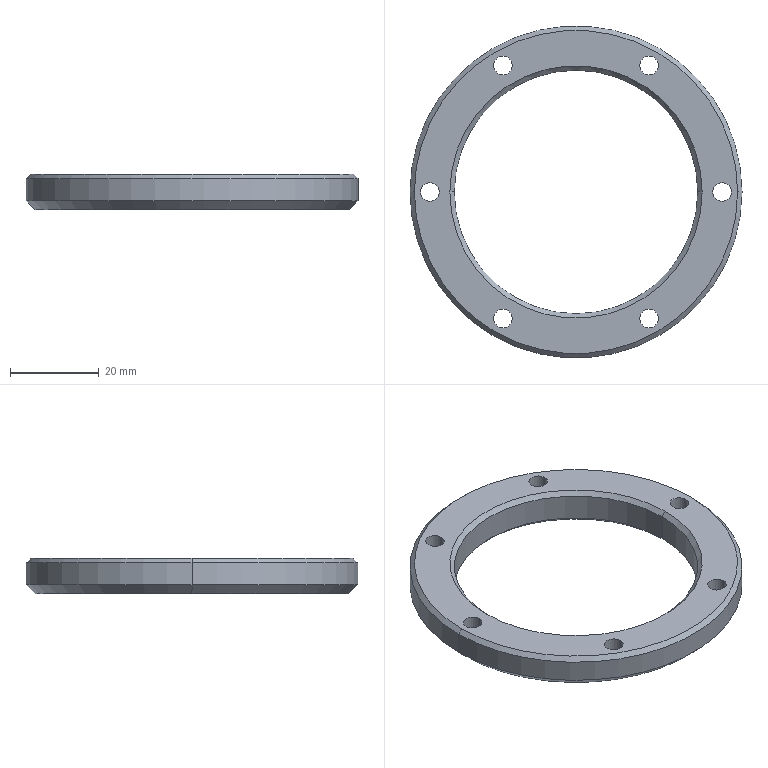Part | STEP file | 10000020571swp000-1 | 1 solid | 26 faces | box 75 x 75 x 8 mm | volume 14917 mm3 | cylinder 16 | cone 8 | plane 2 | commonest cylinder face diameters 4.2 x12 55 x2 75 x2
STEP:
#1=CARTESIAN_POINT('',(-35.5,0.,0.));
#2=VERTEX_POINT('',#1);
#3=CARTESIAN_POINT('',(35.5,0.,0.));
#4=VERTEX_POINT('',#3);
#5=CARTESIAN_POINT('',(0.,0.,0.));
#6=DIRECTION('',(0.,0.,-1.));
#7=DIRECTION('',(1.,0.,0.));
#8=AXIS2_PLACEMENT_3D('',#5,#6,#7);
#9=CIRCLE('',#8,35.5);
#10=EDGE_CURVE('',#2,#4,#9,.T.);
#11=ORIENTED_EDGE('',*,*,#10,.F.);
#12=CARTESIAN_POINT('',(-37.5,0.,2.));
#13=VERTEX_POINT('',#12);
#14=CARTESIAN_POINT('',(-37.5,0.,2.));
#15=DIRECTION('',(-0.7071,0.,0.7071));
#16=VECTOR('',#15,1000.);
#17=LINE('',#14,#16);
#18=EDGE_CURVE('',#2,#13,#17,.T.);
#19=ORIENTED_EDGE('',*,*,#18,.T.);
#20=CARTESIAN_POINT('',(37.5,0.,2.));
#21=VERTEX_POINT('',#20);
#22=CARTESIAN_POINT('',(0.,0.,2.));
#23=DIRECTION('',(0.,0.,1.));
#24=DIRECTION('',(1.,0.,0.));
#25=AXIS2_PLACEMENT_3D('',#22,#23,#24);
#26=CIRCLE('',#25,37.5);
#27=EDGE_CURVE('',#21,#13,#26,.T.);
#28=ORIENTED_EDGE('',*,*,#27,.F.);
#29=CARTESIAN_POINT('',(37.5,0.,2.));
#30=DIRECTION('',(0.7071,0.,0.7071));
#31=VECTOR('',#30,1000.);
#32=LINE('',#29,#31);
#33=EDGE_CURVE('',#4,#21,#32,.T.);
#34=ORIENTED_EDGE('',*,*,#33,.F.);
#35=EDGE_LOOP('',(#11,#19,#28,#34));
#36=FACE_OUTER_BOUND('',#35,.T.);
#37=CARTESIAN_POINT('',(0.,0.,2.));
#38=DIRECTION('',(0.,0.,1.));
#39=DIRECTION('',(1.,0.,0.));
#40=AXIS2_PLACEMENT_3D('',#37,#38,#39);
#41=CONICAL_SURFACE('',#40,37.5,0.7854);
#42=ADVANCED_FACE('',(#36),#41,.T.);
#43=CARTESIAN_POINT('',(-27.5,0.,7.));
#44=VERTEX_POINT('',#43);
#45=CARTESIAN_POINT('',(27.5,0.,7.));
#46=VERTEX_POINT('',#45);
#47=CARTESIAN_POINT('',(0.,0.,7.));
#48=DIRECTION('',(0.,0.,1.));
#49=DIRECTION('',(1.,0.,0.));
#50=AXIS2_PLACEMENT_3D('',#47,#48,#49);
#51=CIRCLE('',#50,27.5);
#52=EDGE_CURVE('',#44,#46,#51,.T.);
#53=ORIENTED_EDGE('',*,*,#52,.F.);
#54=CARTESIAN_POINT('',(-28.5,0.,8.));
#55=VERTEX_POINT('',#54);
#56=CARTESIAN_POINT('',(-27.5,0.,7.));
#57=DIRECTION('',(-0.7071,0.,0.7071));
#58=VECTOR('',#57,1000.);
#59=LINE('',#56,#58);
#60=EDGE_CURVE('',#44,#55,#59,.T.);
#61=ORIENTED_EDGE('',*,*,#60,.T.);
#62=CARTESIAN_POINT('',(28.5,0.,8.));
#63=VERTEX_POINT('',#62);
#64=CARTESIAN_POINT('',(0.,0.,8.));
#65=DIRECTION('',(0.,0.,-1.));
#66=DIRECTION('',(1.,0.,0.));
#67=AXIS2_PLACEMENT_3D('',#64,#65,#66);
#68=CIRCLE('',#67,28.5);
#69=EDGE_CURVE('',#63,#55,#68,.T.);
#70=ORIENTED_EDGE('',*,*,#69,.F.);
#71=CARTESIAN_POINT('',(27.5,0.,7.));
#72=DIRECTION('',(0.7071,0.,0.7071));
#73=VECTOR('',#72,1000.);
#74=LINE('',#71,#73);
#75=EDGE_CURVE('',#46,#63,#74,.T.);
#76=ORIENTED_EDGE('',*,*,#75,.F.);
#77=EDGE_LOOP('',(#53,#61,#70,#76));
#78=FACE_OUTER_BOUND('',#77,.T.);
#79=CARTESIAN_POINT('',(0.,0.,7.));
#80=DIRECTION('',(0.,0.,1.));
#81=DIRECTION('',(1.,0.,0.));
#82=AXIS2_PLACEMENT_3D('',#79,#80,#81);
#83=CONICAL_SURFACE('',#82,27.5,0.7854);
#84=ADVANCED_FACE('',(#78),#83,.F.);
#85=CARTESIAN_POINT('',(27.5,0.,1.));
#86=VERTEX_POINT('',#85);
#87=CARTESIAN_POINT('',(-27.5,0.,1.));
#88=VERTEX_POINT('',#87);
#89=CARTESIAN_POINT('',(0.,0.,1.));
#90=DIRECTION('',(0.,0.,-1.));
#91=DIRECTION('',(1.,0.,0.));
#92=AXIS2_PLACEMENT_3D('',#89,#90,#91);
#93=CIRCLE('',#92,27.5);
#94=EDGE_CURVE('',#86,#88,#93,.T.);
#95=ORIENTED_EDGE('',*,*,#94,.F.);
#96=CARTESIAN_POINT('',(28.5,0.,0.));
#97=VERTEX_POINT('',#96);
#98=CARTESIAN_POINT('',(28.5,0.,0.));
#99=DIRECTION('',(0.7071,0.,-0.7071));
#100=VECTOR('',#99,1000.);
#101=LINE('',#98,#100);
#102=EDGE_CURVE('',#86,#97,#101,.T.);
#103=ORIENTED_EDGE('',*,*,#102,.T.);
#104=CARTESIAN_POINT('',(-28.5,0.,0.));
#105=VERTEX_POINT('',#104);
#106=CARTESIAN_POINT('',(0.,0.,0.));
#107=DIRECTION('',(0.,0.,1.));
#108=DIRECTION('',(1.,0.,0.));
#109=AXIS2_PLACEMENT_3D('',#106,#107,#108);
#110=CIRCLE('',#109,28.5);
#111=EDGE_CURVE('',#105,#97,#110,.T.);
#112=ORIENTED_EDGE('',*,*,#111,.F.);
#113=CARTESIAN_POINT('',(-28.5,0.,0.));
#114=DIRECTION('',(-0.7071,0.,-0.7071));
#115=VECTOR('',#114,1000.);
#116=LINE('',#113,#115);
#117=EDGE_CURVE('',#88,#105,#116,.T.);
#118=ORIENTED_EDGE('',*,*,#117,.F.);
#119=EDGE_LOOP('',(#95,#103,#112,#118));
#120=FACE_OUTER_BOUND('',#119,.T.);
#121=CARTESIAN_POINT('',(0.,0.,0.));
#122=DIRECTION('',(0.,0.,-1.));
#123=DIRECTION('',(-1.,0.,0.));
#124=AXIS2_PLACEMENT_3D('',#121,#122,#123);
#125=CONICAL_SURFACE('',#124,28.5,0.7854);
#126=ADVANCED_FACE('',(#120),#125,.F.);
#127=CARTESIAN_POINT('',(36.5,0.,8.));
#128=VERTEX_POINT('',#127);
#129=CARTESIAN_POINT('',(-36.5,0.,8.));
#130=VERTEX_POINT('',#129);
#131=CARTESIAN_POINT('',(0.,0.,8.));
#132=DIRECTION('',(0.,0.,1.));
#133=DIRECTION('',(1.,0.,0.));
#134=AXIS2_PLACEMENT_3D('',#131,#132,#133);
#135=CIRCLE('',#134,36.5);
#136=EDGE_CURVE('',#128,#130,#135,.T.);
#137=ORIENTED_EDGE('',*,*,#136,.F.);
#138=CARTESIAN_POINT('',(37.5,0.,7.));
#139=VERTEX_POINT('',#138);
#140=CARTESIAN_POINT('',(36.5,0.,8.));
#141=DIRECTION('',(0.7071,0.,-0.7071));
#142=VECTOR('',#141,1000.);
#143=LINE('',#140,#142);
#144=EDGE_CURVE('',#128,#139,#143,.T.);
#145=ORIENTED_EDGE('',*,*,#144,.T.);
#146=CARTESIAN_POINT('',(-37.5,0.,7.));
#147=VERTEX_POINT('',#146);
#148=CARTESIAN_POINT('',(0.,0.,7.));
#149=DIRECTION('',(0.,0.,-1.));
#150=DIRECTION('',(1.,0.,0.));
#151=AXIS2_PLACEMENT_3D('',#148,#149,#150);
#152=CIRCLE('',#151,37.5);
#153=EDGE_CURVE('',#147,#139,#152,.T.);
#154=ORIENTED_EDGE('',*,*,#153,.F.);
#155=CARTESIAN_POINT('',(-36.5,0.,8.));
#156=DIRECTION('',(-0.7071,0.,-0.7071));
#157=VECTOR('',#156,1000.);
#158=LINE('',#155,#157);
#159=EDGE_CURVE('',#130,#147,#158,.T.);
#160=ORIENTED_EDGE('',*,*,#159,.F.);
#161=EDGE_LOOP('',(#137,#145,#154,#160));
#162=FACE_OUTER_BOUND('',#161,.T.);
#163=CARTESIAN_POINT('',(0.,0.,8.));
#164=DIRECTION('',(0.,0.,-1.));
#165=DIRECTION('',(-1.,0.,0.));
#166=AXIS2_PLACEMENT_3D('',#163,#164,#165);
#167=CONICAL_SURFACE('',#166,36.5,0.7854);
#168=ADVANCED_FACE('',(#162),#167,.T.);
#169=CARTESIAN_POINT('',(14.4,28.579,0.));
#170=VERTEX_POINT('',#169);
#171=CARTESIAN_POINT('',(18.6,28.579,0.));
#172=VERTEX_POINT('',#171);
#173=CARTESIAN_POINT('',(16.5,28.579,0.));
#174=DIRECTION('',(0.,0.,1.));
#175=DIRECTION('',(1.,0.,0.));
#176=AXIS2_PLACEMENT_3D('',#173,#174,#175);
#177=CIRCLE('',#176,2.1);
#178=EDGE_CURVE('',#170,#172,#177,.T.);
#179=ORIENTED_EDGE('',*,*,#178,.F.);
#180=CARTESIAN_POINT('',(14.4,28.579,8.));
#181=VERTEX_POINT('',#180);
#182=CARTESIAN_POINT('',(14.4,28.579,8.));
#183=DIRECTION('',(0.,0.,1.));
#184=VECTOR('',#183,1000.);
#185=LINE('',#182,#184);
#186=EDGE_CURVE('',#170,#181,#185,.T.);
#187=ORIENTED_EDGE('',*,*,#186,.T.);
#188=CARTESIAN_POINT('',(18.6,28.579,8.));
#189=VERTEX_POINT('',#188);
#190=CARTESIAN_POINT('',(16.5,28.579,8.));
#191=DIRECTION('',(0.,0.,1.));
#192=DIRECTION('',(1.,0.,0.));
#193=AXIS2_PLACEMENT_3D('',#190,#191,#192);
#194=CIRCLE('',#193,2.1);
#195=EDGE_CURVE('',#181,#189,#194,.T.);
#196=ORIENTED_EDGE('',*,*,#195,.T.);
#197=CARTESIAN_POINT('',(18.6,28.579,8.));
#198=DIRECTION('',(0.,0.,1.));
#199=VECTOR('',#198,1000.);
#200=LINE('',#197,#199);
#201=EDGE_CURVE('',#172,#189,#200,.T.);
#202=ORIENTED_EDGE('',*,*,#201,.F.);
#203=EDGE_LOOP('',(#179,#187,#196,#202));
#204=FACE_OUTER_BOUND('',#203,.T.);
#205=CARTESIAN_POINT('',(16.5,28.579,8.));
#206=DIRECTION('',(0.,0.,1.));
#207=DIRECTION('',(1.,0.,0.));
#208=AXIS2_PLACEMENT_3D('',#205,#206,#207);
#209=CYLINDRICAL_SURFACE('',#208,2.1);
#210=ADVANCED_FACE('',(#204),#209,.F.);
#211=CARTESIAN_POINT('',(-18.6,28.579,0.));
#212=VERTEX_POINT('',#211);
#213=CARTESIAN_POINT('',(-14.4,28.579,0.));
#214=VERTEX_POINT('',#213);
#215=CARTESIAN_POINT('',(-16.5,28.579,0.));
#216=DIRECTION('',(0.,0.,1.));
#217=DIRECTION('',(1.,0.,0.));
#218=AXIS2_PLACEMENT_3D('',#215,#216,#217);
#219=CIRCLE('',#218,2.1);
#220=EDGE_CURVE('',#212,#214,#219,.T.);
#221=ORIENTED_EDGE('',*,*,#220,.F.);
#222=CARTESIAN_POINT('',(-18.6,28.579,8.));
#223=VERTEX_POINT('',#222);
#224=CARTESIAN_POINT('',(-18.6,28.579,8.));
#225=DIRECTION('',(0.,0.,1.));
#226=VECTOR('',#225,1000.);
#227=LINE('',#224,#226);
#228=EDGE_CURVE('',#212,#223,#227,.T.);
#229=ORIENTED_EDGE('',*,*,#228,.T.);
#230=CARTESIAN_POINT('',(-14.4,28.579,8.));
#231=VERTEX_POINT('',#230);
#232=CARTESIAN_POINT('',(-16.5,28.579,8.));
#233=DIRECTION('',(0.,0.,1.));
#234=DIRECTION('',(1.,0.,0.));
#235=AXIS2_PLACEMENT_3D('',#232,#233,#234);
#236=CIRCLE('',#235,2.1);
#237=EDGE_CURVE('',#223,#231,#236,.T.);
#238=ORIENTED_EDGE('',*,*,#237,.T.);
#239=CARTESIAN_POINT('',(-14.4,28.579,8.));
#240=DIRECTION('',(0.,0.,1.));
#241=VECTOR('',#240,1000.);
#242=LINE('',#239,#241);
#243=EDGE_CURVE('',#214,#231,#242,.T.);
#244=ORIENTED_EDGE('',*,*,#243,.F.);
#245=EDGE_LOOP('',(#221,#229,#238,#244));
#246=FACE_OUTER_BOUND('',#245,.T.);
#247=CARTESIAN_POINT('',(-16.5,28.579,8.));
#248=DIRECTION('',(0.,0.,1.));
#249=DIRECTION('',(1.,0.,0.));
#250=AXIS2_PLACEMENT_3D('',#247,#248,#249);
#251=CYLINDRICAL_SURFACE('',#250,2.1);
#252=ADVANCED_FACE('',(#246),#251,.F.);
#253=CARTESIAN_POINT('',(-35.1,0.,0.));
#254=VERTEX_POINT('',#253);
#255=CARTESIAN_POINT('',(-30.9,0.,0.));
#256=VERTEX_POINT('',#255);
#257=CARTESIAN_POINT('',(-33.,0.,0.));
#258=DIRECTION('',(0.,0.,1.));
#259=DIRECTION('',(1.,0.,0.));
#260=AXIS2_PLACEMENT_3D('',#257,#258,#259);
#261=CIRCLE('',#260,2.1);
#262=EDGE_CURVE('',#254,#256,#261,.T.);
#263=ORIENTED_EDGE('',*,*,#262,.F.);
#264=CARTESIAN_POINT('',(-35.1,0.,8.));
#265=VERTEX_POINT('',#264);
#266=CARTESIAN_POINT('',(-35.1,0.,8.));
#267=DIRECTION('',(0.,0.,1.));
#268=VECTOR('',#267,1000.);
#269=LINE('',#266,#268);
#270=EDGE_CURVE('',#254,#265,#269,.T.);
#271=ORIENTED_EDGE('',*,*,#270,.T.);
#272=CARTESIAN_POINT('',(-30.9,0.,8.));
#273=VERTEX_POINT('',#272);
#274=CARTESIAN_POINT('',(-33.,0.,8.));
#275=DIRECTION('',(0.,0.,1.));
#276=DIRECTION('',(1.,0.,0.));
#277=AXIS2_PLACEMENT_3D('',#274,#275,#276);
#278=CIRCLE('',#277,2.1);
#279=EDGE_CURVE('',#265,#273,#278,.T.);
#280=ORIENTED_EDGE('',*,*,#279,.T.);
#281=CARTESIAN_POINT('',(-30.9,0.,8.));
#282=DIRECTION('',(0.,0.,1.));
#283=VECTOR('',#282,1000.);
#284=LINE('',#281,#283);
#285=EDGE_CURVE('',#256,#273,#284,.T.);
#286=ORIENTED_EDGE('',*,*,#285,.F.);
#287=EDGE_LOOP('',(#263,#271,#280,#286));
#288=FACE_OUTER_BOUND('',#287,.T.);
#289=CARTESIAN_POINT('',(-33.,0.,8.));
#290=DIRECTION('',(0.,0.,1.));
#291=DIRECTION('',(1.,0.,0.));
#292=AXIS2_PLACEMENT_3D('',#289,#290,#291);
#293=CYLINDRICAL_SURFACE('',#292,2.1);
#294=ADVANCED_FACE('',(#288),#293,.F.);
#295=CARTESIAN_POINT('',(-18.6,-28.579,0.));
#296=VERTEX_POINT('',#295);
#297=CARTESIAN_POINT('',(-14.4,-28.579,0.));
#298=VERTEX_POINT('',#297);
#299=CARTESIAN_POINT('',(-16.5,-28.579,0.));
#300=DIRECTION('',(0.,0.,1.));
#301=DIRECTION('',(1.,0.,0.));
#302=AXIS2_PLACEMENT_3D('',#299,#300,#301);
#303=CIRCLE('',#302,2.1);
#304=EDGE_CURVE('',#296,#298,#303,.T.);
#305=ORIENTED_EDGE('',*,*,#304,.F.);
#306=CARTESIAN_POINT('',(-18.6,-28.579,8.));
#307=VERTEX_POINT('',#306);
#308=CARTESIAN_POINT('',(-18.6,-28.579,8.));
#309=DIRECTION('',(0.,0.,1.));
#310=VECTOR('',#309,1000.);
#311=LINE('',#308,#310);
#312=EDGE_CURVE('',#296,#307,#311,.T.);
#313=ORIENTED_EDGE('',*,*,#312,.T.);
#314=CARTESIAN_POINT('',(-14.4,-28.579,8.));
#315=VERTEX_POINT('',#314);
#316=CARTESIAN_POINT('',(-16.5,-28.579,8.));
#317=DIRECTION('',(0.,0.,1.));
#318=DIRECTION('',(1.,0.,0.));
#319=AXIS2_PLACEMENT_3D('',#316,#317,#318);
#320=CIRCLE('',#319,2.1);
#321=EDGE_CURVE('',#307,#315,#320,.T.);
#322=ORIENTED_EDGE('',*,*,#321,.T.);
#323=CARTESIAN_POINT('',(-14.4,-28.579,8.));
#324=DIRECTION('',(0.,0.,1.));
#325=VECTOR('',#324,1000.);
#326=LINE('',#323,#325);
#327=EDGE_CURVE('',#298,#315,#326,.T.);
#328=ORIENTED_EDGE('',*,*,#327,.F.);
#329=EDGE_LOOP('',(#305,#313,#322,#328));
#330=FACE_OUTER_BOUND('',#329,.T.);
#331=CARTESIAN_POINT('',(-16.5,-28.579,8.));
#332=DIRECTION('',(0.,0.,1.));
#333=DIRECTION('',(1.,0.,0.));
#334=AXIS2_PLACEMENT_3D('',#331,#332,#333);
#335=CYLINDRICAL_SURFACE('',#334,2.1);
#336=ADVANCED_FACE('',(#330),#335,.F.);
#337=CARTESIAN_POINT('',(14.4,-28.579,0.));
#338=VERTEX_POINT('',#337);
#339=CARTESIAN_POINT('',(18.6,-28.579,0.));
#340=VERTEX_POINT('',#339);
#341=CARTESIAN_POINT('',(16.5,-28.579,0.));
#342=DIRECTION('',(0.,0.,1.));
#343=DIRECTION('',(1.,0.,0.));
#344=AXIS2_PLACEMENT_3D('',#341,#342,#343);
#345=CIRCLE('',#344,2.1);
#346=EDGE_CURVE('',#338,#340,#345,.T.);
#347=ORIENTED_EDGE('',*,*,#346,.F.);
#348=CARTESIAN_POINT('',(14.4,-28.579,8.));
#349=VERTEX_POINT('',#348);
#350=CARTESIAN_POINT('',(14.4,-28.579,8.));
#351=DIRECTION('',(0.,0.,1.));
#352=VECTOR('',#351,1000.);
#353=LINE('',#350,#352);
#354=EDGE_CURVE('',#338,#349,#353,.T.);
#355=ORIENTED_EDGE('',*,*,#354,.T.);
#356=CARTESIAN_POINT('',(18.6,-28.579,8.));
#357=VERTEX_POINT('',#356);
#358=CARTESIAN_POINT('',(16.5,-28.579,8.));
#359=DIRECTION('',(0.,0.,1.));
#360=DIRECTION('',(1.,0.,0.));
#361=AXIS2_PLACEMENT_3D('',#358,#359,#360);
#362=CIRCLE('',#361,2.1);
#363=EDGE_CURVE('',#349,#357,#362,.T.);
#364=ORIENTED_EDGE('',*,*,#363,.T.);
#365=CARTESIAN_POINT('',(18.6,-28.579,8.));
#366=DIRECTION('',(0.,0.,1.));
#367=VECTOR('',#366,1000.);
#368=LINE('',#365,#367);
#369=EDGE_CURVE('',#340,#357,#368,.T.);
#370=ORIENTED_EDGE('',*,*,#369,.F.);
#371=EDGE_LOOP('',(#347,#355,#364,#370));
#372=FACE_OUTER_BOUND('',#371,.T.);
#373=CARTESIAN_POINT('',(16.5,-28.579,8.));
#374=DIRECTION('',(0.,0.,1.));
#375=DIRECTION('',(1.,0.,0.));
#376=AXIS2_PLACEMENT_3D('',#373,#374,#375);
#377=CYLINDRICAL_SURFACE('',#376,2.1);
#378=ADVANCED_FACE('',(#372),#377,.F.);
#379=CARTESIAN_POINT('',(30.9,0.,0.));
#380=VERTEX_POINT('',#379);
#381=CARTESIAN_POINT('',(35.1,0.,0.));
#382=VERTEX_POINT('',#381);
#383=CARTESIAN_POINT('',(33.,0.,0.));
#384=DIRECTION('',(0.,0.,1.));
#385=DIRECTION('',(1.,0.,0.));
#386=AXIS2_PLACEMENT_3D('',#383,#384,#385);
#387=CIRCLE('',#386,2.1);
#388=EDGE_CURVE('',#380,#382,#387,.T.);
#389=ORIENTED_EDGE('',*,*,#388,.F.);
#390=CARTESIAN_POINT('',(30.9,0.,8.));
#391=VERTEX_POINT('',#390);
#392=CARTESIAN_POINT('',(30.9,0.,8.));
#393=DIRECTION('',(0.,0.,1.));
#394=VECTOR('',#393,1000.);
#395=LINE('',#392,#394);
#396=EDGE_CURVE('',#380,#391,#395,.T.);
#397=ORIENTED_EDGE('',*,*,#396,.T.);
#398=CARTESIAN_POINT('',(35.1,0.,8.));
#399=VERTEX_POINT('',#398);
#400=CARTESIAN_POINT('',(33.,0.,8.));
#401=DIRECTION('',(0.,0.,1.));
#402=DIRECTION('',(1.,0.,0.));
#403=AXIS2_PLACEMENT_3D('',#400,#401,#402);
#404=CIRCLE('',#403,2.1);
#405=EDGE_CURVE('',#391,#399,#404,.T.);
#406=ORIENTED_EDGE('',*,*,#405,.T.);
#407=CARTESIAN_POINT('',(35.1,0.,8.));
#408=DIRECTION('',(0.,0.,1.));
#409=VECTOR('',#408,1000.);
#410=LINE('',#407,#409);
#411=EDGE_CURVE('',#382,#399,#410,.T.);
#412=ORIENTED_EDGE('',*,*,#411,.F.);
#413=EDGE_LOOP('',(#389,#397,#406,#412));
#414=FACE_OUTER_BOUND('',#413,.T.);
#415=CARTESIAN_POINT('',(33.,0.,8.));
#416=DIRECTION('',(0.,0.,1.));
#417=DIRECTION('',(1.,0.,0.));
#418=AXIS2_PLACEMENT_3D('',#415,#416,#417);
#419=CYLINDRICAL_SURFACE('',#418,2.1);
#420=ADVANCED_FACE('',(#414),#419,.F.);
#421=ORIENTED_EDGE('',*,*,#52,.T.);
#422=CARTESIAN_POINT('',(27.5,0.,8.));
#423=DIRECTION('',(0.,0.,-1.));
#424=VECTOR('',#423,1000.);
#425=LINE('',#422,#424);
#426=EDGE_CURVE('',#46,#86,#425,.T.);
#427=ORIENTED_EDGE('',*,*,#426,.T.);
#428=ORIENTED_EDGE('',*,*,#94,.T.);
#429=CARTESIAN_POINT('',(-27.5,0.,8.));
#430=DIRECTION('',(0.,0.,-1.));
#431=VECTOR('',#430,1000.);
#432=LINE('',#429,#431);
#433=EDGE_CURVE('',#44,#88,#432,.T.);
#434=ORIENTED_EDGE('',*,*,#433,.F.);
#435=EDGE_LOOP('',(#421,#427,#428,#434));
#436=FACE_OUTER_BOUND('',#435,.T.);
#437=CARTESIAN_POINT('',(0.,0.,8.));
#438=DIRECTION('',(0.,0.,-1.));
#439=DIRECTION('',(-1.,0.,0.));
#440=AXIS2_PLACEMENT_3D('',#437,#438,#439);
#441=CYLINDRICAL_SURFACE('',#440,27.5);
#442=ADVANCED_FACE('',(#436),#441,.F.);
#443=ORIENTED_EDGE('',*,*,#153,.T.);
#444=CARTESIAN_POINT('',(37.5,0.,8.));
#445=DIRECTION('',(0.,0.,-1.));
#446=VECTOR('',#445,1000.);
#447=LINE('',#444,#446);
#448=EDGE_CURVE('',#139,#21,#447,.T.);
#449=ORIENTED_EDGE('',*,*,#448,.T.);
#450=ORIENTED_EDGE('',*,*,#27,.T.);
#451=CARTESIAN_POINT('',(-37.5,0.,8.));
#452=DIRECTION('',(0.,0.,-1.));
#453=VECTOR('',#452,1000.);
#454=LINE('',#451,#453);
#455=EDGE_CURVE('',#147,#13,#454,.T.);
#456=ORIENTED_EDGE('',*,*,#455,.F.);
#457=EDGE_LOOP('',(#443,#449,#450,#456));
#458=FACE_OUTER_BOUND('',#457,.T.);
#459=CARTESIAN_POINT('',(0.,0.,8.));
#460=DIRECTION('',(0.,0.,-1.));
#461=DIRECTION('',(-1.,0.,0.));
#462=AXIS2_PLACEMENT_3D('',#459,#460,#461);
#463=CYLINDRICAL_SURFACE('',#462,37.5);
#464=ADVANCED_FACE('',(#458),#463,.T.);
#465=CARTESIAN_POINT('',(0.,0.,8.));
#466=DIRECTION('',(0.,0.,1.));
#467=DIRECTION('',(1.,0.,0.));
#468=AXIS2_PLACEMENT_3D('',#465,#466,#467);
#469=CIRCLE('',#468,36.5);
#470=EDGE_CURVE('',#130,#128,#469,.T.);
#471=ORIENTED_EDGE('',*,*,#470,.T.);
#472=ORIENTED_EDGE('',*,*,#136,.T.);
#473=EDGE_LOOP('',(#471,#472));
#474=FACE_OUTER_BOUND('',#473,.T.);
#475=ORIENTED_EDGE('',*,*,#69,.T.);
#476=CARTESIAN_POINT('',(0.,0.,8.));
#477=DIRECTION('',(0.,0.,-1.));
#478=DIRECTION('',(1.,0.,0.));
#479=AXIS2_PLACEMENT_3D('',#476,#477,#478);
#480=CIRCLE('',#479,28.5);
#481=EDGE_CURVE('',#55,#63,#480,.T.);
#482=ORIENTED_EDGE('',*,*,#481,.T.);
#483=EDGE_LOOP('',(#475,#482));
#484=FACE_BOUND('',#483,.T.);
#485=CARTESIAN_POINT('',(16.5,28.579,8.));
#486=DIRECTION('',(0.,0.,1.));
#487=DIRECTION('',(1.,0.,0.));
#488=AXIS2_PLACEMENT_3D('',#485,#486,#487);
#489=CIRCLE('',#488,2.1);
#490=EDGE_CURVE('',#189,#181,#489,.T.);
#491=ORIENTED_EDGE('',*,*,#490,.F.);
#492=ORIENTED_EDGE('',*,*,#195,.F.);
#493=EDGE_LOOP('',(#491,#492));
#494=FACE_BOUND('',#493,.T.);
#495=CARTESIAN_POINT('',(-16.5,28.579,8.));
#496=DIRECTION('',(0.,0.,1.));
#497=DIRECTION('',(1.,0.,0.));
#498=AXIS2_PLACEMENT_3D('',#495,#496,#497);
#499=CIRCLE('',#498,2.1);
#500=EDGE_CURVE('',#231,#223,#499,.T.);
#501=ORIENTED_EDGE('',*,*,#500,.F.);
#502=ORIENTED_EDGE('',*,*,#237,.F.);
#503=EDGE_LOOP('',(#501,#502));
#504=FACE_BOUND('',#503,.T.);
#505=CARTESIAN_POINT('',(-33.,0.,8.));
#506=DIRECTION('',(0.,0.,1.));
#507=DIRECTION('',(1.,0.,0.));
#508=AXIS2_PLACEMENT_3D('',#505,#506,#507);
#509=CIRCLE('',#508,2.1);
#510=EDGE_CURVE('',#273,#265,#509,.T.);
#511=ORIENTED_EDGE('',*,*,#510,.F.);
#512=ORIENTED_EDGE('',*,*,#279,.F.);
#513=EDGE_LOOP('',(#511,#512));
#514=FACE_BOUND('',#513,.T.);
#515=CARTESIAN_POINT('',(-16.5,-28.579,8.));
#516=DIRECTION('',(0.,0.,1.));
#517=DIRECTION('',(1.,0.,0.));
#518=AXIS2_PLACEMENT_3D('',#515,#516,#517);
#519=CIRCLE('',#518,2.1);
#520=EDGE_CURVE('',#315,#307,#519,.T.);
#521=ORIENTED_EDGE('',*,*,#520,.F.);
#522=ORIENTED_EDGE('',*,*,#321,.F.);
#523=EDGE_LOOP('',(#521,#522));
#524=FACE_BOUND('',#523,.T.);
#525=CARTESIAN_POINT('',(16.5,-28.579,8.));
#526=DIRECTION('',(0.,0.,1.));
#527=DIRECTION('',(1.,0.,0.));
#528=AXIS2_PLACEMENT_3D('',#525,#526,#527);
#529=CIRCLE('',#528,2.1);
#530=EDGE_CURVE('',#357,#349,#529,.T.);
#531=ORIENTED_EDGE('',*,*,#530,.F.);
#532=ORIENTED_EDGE('',*,*,#363,.F.);
#533=EDGE_LOOP('',(#531,#532));
#534=FACE_BOUND('',#533,.T.);
#535=CARTESIAN_POINT('',(33.,0.,8.));
#536=DIRECTION('',(0.,0.,1.));
#537=DIRECTION('',(1.,0.,0.));
#538=AXIS2_PLACEMENT_3D('',#535,#536,#537);
#539=CIRCLE('',#538,2.1);
#540=EDGE_CURVE('',#399,#391,#539,.T.);
#541=ORIENTED_EDGE('',*,*,#540,.F.);
#542=ORIENTED_EDGE('',*,*,#405,.F.);
#543=EDGE_LOOP('',(#541,#542));
#544=FACE_BOUND('',#543,.T.);
#545=CARTESIAN_POINT('',(0.,0.,8.));
#546=DIRECTION('',(0.,0.,1.));
#547=DIRECTION('',(1.,0.,0.));
#548=AXIS2_PLACEMENT_3D('',#545,#546,#547);
#549=PLANE('',#548);
#550=ADVANCED_FACE('',(#474,#484,#494,#504,#514,#524,#534,#544),#549,.T.);
#551=CARTESIAN_POINT('',(0.,0.,0.));
#552=DIRECTION('',(0.,0.,-1.));
#553=DIRECTION('',(1.,0.,0.));
#554=AXIS2_PLACEMENT_3D('',#551,#552,#553);
#555=CIRCLE('',#554,35.5);
#556=EDGE_CURVE('',#4,#2,#555,.T.);
#557=ORIENTED_EDGE('',*,*,#556,.T.);
#558=ORIENTED_EDGE('',*,*,#10,.T.);
#559=EDGE_LOOP('',(#557,#558));
#560=FACE_OUTER_BOUND('',#559,.T.);
#561=ORIENTED_EDGE('',*,*,#111,.T.);
#562=CARTESIAN_POINT('',(0.,0.,0.));
#563=DIRECTION('',(0.,0.,1.));
#564=DIRECTION('',(1.,0.,0.));
#565=AXIS2_PLACEMENT_3D('',#562,#563,#564);
#566=CIRCLE('',#565,28.5);
#567=EDGE_CURVE('',#97,#105,#566,.T.);
#568=ORIENTED_EDGE('',*,*,#567,.T.);
#569=EDGE_LOOP('',(#561,#568));
#570=FACE_BOUND('',#569,.T.);
#571=CARTESIAN_POINT('',(16.5,28.579,0.));
#572=DIRECTION('',(0.,0.,1.));
#573=DIRECTION('',(1.,0.,0.));
#574=AXIS2_PLACEMENT_3D('',#571,#572,#573);
#575=CIRCLE('',#574,2.1);
#576=EDGE_CURVE('',#172,#170,#575,.T.);
#577=ORIENTED_EDGE('',*,*,#576,.T.);
#578=ORIENTED_EDGE('',*,*,#178,.T.);
#579=EDGE_LOOP('',(#577,#578));
#580=FACE_BOUND('',#579,.T.);
#581=CARTESIAN_POINT('',(-16.5,28.579,0.));
#582=DIRECTION('',(0.,0.,1.));
#583=DIRECTION('',(1.,0.,0.));
#584=AXIS2_PLACEMENT_3D('',#581,#582,#583);
#585=CIRCLE('',#584,2.1);
#586=EDGE_CURVE('',#214,#212,#585,.T.);
#587=ORIENTED_EDGE('',*,*,#586,.T.);
#588=ORIENTED_EDGE('',*,*,#220,.T.);
#589=EDGE_LOOP('',(#587,#588));
#590=FACE_BOUND('',#589,.T.);
#591=CARTESIAN_POINT('',(-33.,0.,0.));
#592=DIRECTION('',(0.,0.,1.));
#593=DIRECTION('',(1.,0.,0.));
#594=AXIS2_PLACEMENT_3D('',#591,#592,#593);
#595=CIRCLE('',#594,2.1);
#596=EDGE_CURVE('',#256,#254,#595,.T.);
#597=ORIENTED_EDGE('',*,*,#596,.T.);
#598=ORIENTED_EDGE('',*,*,#262,.T.);
#599=EDGE_LOOP('',(#597,#598));
#600=FACE_BOUND('',#599,.T.);
#601=CARTESIAN_POINT('',(-16.5,-28.579,0.));
#602=DIRECTION('',(0.,0.,1.));
#603=DIRECTION('',(1.,0.,0.));
#604=AXIS2_PLACEMENT_3D('',#601,#602,#603);
#605=CIRCLE('',#604,2.1);
#606=EDGE_CURVE('',#298,#296,#605,.T.);
#607=ORIENTED_EDGE('',*,*,#606,.T.);
#608=ORIENTED_EDGE('',*,*,#304,.T.);
#609=EDGE_LOOP('',(#607,#608));
#610=FACE_BOUND('',#609,.T.);
#611=CARTESIAN_POINT('',(16.5,-28.579,0.));
#612=DIRECTION('',(0.,0.,1.));
#613=DIRECTION('',(1.,0.,0.));
#614=AXIS2_PLACEMENT_3D('',#611,#612,#613);
#615=CIRCLE('',#614,2.1);
#616=EDGE_CURVE('',#340,#338,#615,.T.);
#617=ORIENTED_EDGE('',*,*,#616,.T.);
#618=ORIENTED_EDGE('',*,*,#346,.T.);
#619=EDGE_LOOP('',(#617,#618));
#620=FACE_BOUND('',#619,.T.);
#621=CARTESIAN_POINT('',(33.,0.,0.));
#622=DIRECTION('',(0.,0.,1.));
#623=DIRECTION('',(1.,0.,0.));
#624=AXIS2_PLACEMENT_3D('',#621,#622,#623);
#625=CIRCLE('',#624,2.1);
#626=EDGE_CURVE('',#382,#380,#625,.T.);
#627=ORIENTED_EDGE('',*,*,#626,.T.);
#628=ORIENTED_EDGE('',*,*,#388,.T.);
#629=EDGE_LOOP('',(#627,#628));
#630=FACE_BOUND('',#629,.T.);
#631=CARTESIAN_POINT('',(0.,0.,0.));
#632=DIRECTION('',(0.,0.,1.));
#633=DIRECTION('',(1.,0.,0.));
#634=AXIS2_PLACEMENT_3D('',#631,#632,#633);
#635=PLANE('',#634);
#636=ADVANCED_FACE('',(#560,#570,#580,#590,#600,#610,#620,#630),#635,.F.);
#637=ORIENTED_EDGE('',*,*,#448,.F.);
#638=CARTESIAN_POINT('',(0.,0.,7.));
#639=DIRECTION('',(0.,0.,-1.));
#640=DIRECTION('',(1.,0.,0.));
#641=AXIS2_PLACEMENT_3D('',#638,#639,#640);
#642=CIRCLE('',#641,37.5);
#643=EDGE_CURVE('',#139,#147,#642,.T.);
#644=ORIENTED_EDGE('',*,*,#643,.T.);
#645=ORIENTED_EDGE('',*,*,#455,.T.);
#646=CARTESIAN_POINT('',(0.,0.,2.));
#647=DIRECTION('',(0.,0.,1.));
#648=DIRECTION('',(1.,0.,0.));
#649=AXIS2_PLACEMENT_3D('',#646,#647,#648);
#650=CIRCLE('',#649,37.5);
#651=EDGE_CURVE('',#13,#21,#650,.T.);
#652=ORIENTED_EDGE('',*,*,#651,.T.);
#653=EDGE_LOOP('',(#637,#644,#645,#652));
#654=FACE_OUTER_BOUND('',#653,.T.);
#655=CARTESIAN_POINT('',(0.,0.,8.));
#656=DIRECTION('',(0.,0.,-1.));
#657=DIRECTION('',(-1.,0.,0.));
#658=AXIS2_PLACEMENT_3D('',#655,#656,#657);
#659=CYLINDRICAL_SURFACE('',#658,37.5);
#660=ADVANCED_FACE('',(#654),#659,.T.);
#661=ORIENTED_EDGE('',*,*,#426,.F.);
#662=CARTESIAN_POINT('',(0.,0.,7.));
#663=DIRECTION('',(0.,0.,1.));
#664=DIRECTION('',(1.,0.,0.));
#665=AXIS2_PLACEMENT_3D('',#662,#663,#664);
#666=CIRCLE('',#665,27.5);
#667=EDGE_CURVE('',#46,#44,#666,.T.);
#668=ORIENTED_EDGE('',*,*,#667,.T.);
#669=ORIENTED_EDGE('',*,*,#433,.T.);
#670=CARTESIAN_POINT('',(0.,0.,1.));
#671=DIRECTION('',(0.,0.,-1.));
#672=DIRECTION('',(1.,0.,0.));
#673=AXIS2_PLACEMENT_3D('',#670,#671,#672);
#674=CIRCLE('',#673,27.5);
#675=EDGE_CURVE('',#88,#86,#674,.T.);
#676=ORIENTED_EDGE('',*,*,#675,.T.);
#677=EDGE_LOOP('',(#661,#668,#669,#676));
#678=FACE_OUTER_BOUND('',#677,.T.);
#679=CARTESIAN_POINT('',(0.,0.,8.));
#680=DIRECTION('',(0.,0.,-1.));
#681=DIRECTION('',(-1.,0.,0.));
#682=AXIS2_PLACEMENT_3D('',#679,#680,#681);
#683=CYLINDRICAL_SURFACE('',#682,27.5);
#684=ADVANCED_FACE('',(#678),#683,.F.);
#685=ORIENTED_EDGE('',*,*,#396,.F.);
#686=ORIENTED_EDGE('',*,*,#626,.F.);
#687=ORIENTED_EDGE('',*,*,#411,.T.);
#688=ORIENTED_EDGE('',*,*,#540,.T.);
#689=EDGE_LOOP('',(#685,#686,#687,#688));
#690=FACE_OUTER_BOUND('',#689,.T.);
#691=CARTESIAN_POINT('',(33.,0.,8.));
#692=DIRECTION('',(0.,0.,1.));
#693=DIRECTION('',(1.,0.,0.));
#694=AXIS2_PLACEMENT_3D('',#691,#692,#693);
#695=CYLINDRICAL_SURFACE('',#694,2.1);
#696=ADVANCED_FACE('',(#690),#695,.F.);
#697=ORIENTED_EDGE('',*,*,#354,.F.);
#698=ORIENTED_EDGE('',*,*,#616,.F.);
#699=ORIENTED_EDGE('',*,*,#369,.T.);
#700=ORIENTED_EDGE('',*,*,#530,.T.);
#701=EDGE_LOOP('',(#697,#698,#699,#700));
#702=FACE_OUTER_BOUND('',#701,.T.);
#703=CARTESIAN_POINT('',(16.5,-28.579,8.));
#704=DIRECTION('',(0.,0.,1.));
#705=DIRECTION('',(1.,0.,0.));
#706=AXIS2_PLACEMENT_3D('',#703,#704,#705);
#707=CYLINDRICAL_SURFACE('',#706,2.1);
#708=ADVANCED_FACE('',(#702),#707,.F.);
#709=ORIENTED_EDGE('',*,*,#312,.F.);
#710=ORIENTED_EDGE('',*,*,#606,.F.);
#711=ORIENTED_EDGE('',*,*,#327,.T.);
#712=ORIENTED_EDGE('',*,*,#520,.T.);
#713=EDGE_LOOP('',(#709,#710,#711,#712));
#714=FACE_OUTER_BOUND('',#713,.T.);
#715=CARTESIAN_POINT('',(-16.5,-28.579,8.));
#716=DIRECTION('',(0.,0.,1.));
#717=DIRECTION('',(1.,0.,0.));
#718=AXIS2_PLACEMENT_3D('',#715,#716,#717);
#719=CYLINDRICAL_SURFACE('',#718,2.1);
#720=ADVANCED_FACE('',(#714),#719,.F.);
#721=ORIENTED_EDGE('',*,*,#270,.F.);
#722=ORIENTED_EDGE('',*,*,#596,.F.);
#723=ORIENTED_EDGE('',*,*,#285,.T.);
#724=ORIENTED_EDGE('',*,*,#510,.T.);
#725=EDGE_LOOP('',(#721,#722,#723,#724));
#726=FACE_OUTER_BOUND('',#725,.T.);
#727=CARTESIAN_POINT('',(-33.,0.,8.));
#728=DIRECTION('',(0.,0.,1.));
#729=DIRECTION('',(1.,0.,0.));
#730=AXIS2_PLACEMENT_3D('',#727,#728,#729);
#731=CYLINDRICAL_SURFACE('',#730,2.1);
#732=ADVANCED_FACE('',(#726),#731,.F.);
#733=ORIENTED_EDGE('',*,*,#228,.F.);
#734=ORIENTED_EDGE('',*,*,#586,.F.);
#735=ORIENTED_EDGE('',*,*,#243,.T.);
#736=ORIENTED_EDGE('',*,*,#500,.T.);
#737=EDGE_LOOP('',(#733,#734,#735,#736));
#738=FACE_OUTER_BOUND('',#737,.T.);
#739=CARTESIAN_POINT('',(-16.5,28.579,8.));
#740=DIRECTION('',(0.,0.,1.));
#741=DIRECTION('',(1.,0.,0.));
#742=AXIS2_PLACEMENT_3D('',#739,#740,#741);
#743=CYLINDRICAL_SURFACE('',#742,2.1);
#744=ADVANCED_FACE('',(#738),#743,.F.);
#745=ORIENTED_EDGE('',*,*,#186,.F.);
#746=ORIENTED_EDGE('',*,*,#576,.F.);
#747=ORIENTED_EDGE('',*,*,#201,.T.);
#748=ORIENTED_EDGE('',*,*,#490,.T.);
#749=EDGE_LOOP('',(#745,#746,#747,#748));
#750=FACE_OUTER_BOUND('',#749,.T.);
#751=CARTESIAN_POINT('',(16.5,28.579,8.));
#752=DIRECTION('',(0.,0.,1.));
#753=DIRECTION('',(1.,0.,0.));
#754=AXIS2_PLACEMENT_3D('',#751,#752,#753);
#755=CYLINDRICAL_SURFACE('',#754,2.1);
#756=ADVANCED_FACE('',(#750),#755,.F.);
#757=ORIENTED_EDGE('',*,*,#144,.F.);
#758=ORIENTED_EDGE('',*,*,#470,.F.);
#759=ORIENTED_EDGE('',*,*,#159,.T.);
#760=ORIENTED_EDGE('',*,*,#643,.F.);
#761=EDGE_LOOP('',(#757,#758,#759,#760));
#762=FACE_OUTER_BOUND('',#761,.T.);
#763=CARTESIAN_POINT('',(0.,0.,8.));
#764=DIRECTION('',(0.,0.,-1.));
#765=DIRECTION('',(-1.,0.,0.));
#766=AXIS2_PLACEMENT_3D('',#763,#764,#765);
#767=CONICAL_SURFACE('',#766,36.5,0.7854);
#768=ADVANCED_FACE('',(#762),#767,.T.);
#769=ORIENTED_EDGE('',*,*,#102,.F.);
#770=ORIENTED_EDGE('',*,*,#675,.F.);
#771=ORIENTED_EDGE('',*,*,#117,.T.);
#772=ORIENTED_EDGE('',*,*,#567,.F.);
#773=EDGE_LOOP('',(#769,#770,#771,#772));
#774=FACE_OUTER_BOUND('',#773,.T.);
#775=CARTESIAN_POINT('',(0.,0.,0.));
#776=DIRECTION('',(0.,0.,-1.));
#777=DIRECTION('',(-1.,0.,0.));
#778=AXIS2_PLACEMENT_3D('',#775,#776,#777);
#779=CONICAL_SURFACE('',#778,28.5,0.7854);
#780=ADVANCED_FACE('',(#774),#779,.F.);
#781=ORIENTED_EDGE('',*,*,#60,.F.);
#782=ORIENTED_EDGE('',*,*,#667,.F.);
#783=ORIENTED_EDGE('',*,*,#75,.T.);
#784=ORIENTED_EDGE('',*,*,#481,.F.);
#785=EDGE_LOOP('',(#781,#782,#783,#784));
#786=FACE_OUTER_BOUND('',#785,.T.);
#787=CARTESIAN_POINT('',(0.,0.,7.));
#788=DIRECTION('',(0.,0.,1.));
#789=DIRECTION('',(1.,0.,0.));
#790=AXIS2_PLACEMENT_3D('',#787,#788,#789);
#791=CONICAL_SURFACE('',#790,27.5,0.7854);
#792=ADVANCED_FACE('',(#786),#791,.F.);
#793=ORIENTED_EDGE('',*,*,#18,.F.);
#794=ORIENTED_EDGE('',*,*,#556,.F.);
#795=ORIENTED_EDGE('',*,*,#33,.T.);
#796=ORIENTED_EDGE('',*,*,#651,.F.);
#797=EDGE_LOOP('',(#793,#794,#795,#796));
#798=FACE_OUTER_BOUND('',#797,.T.);
#799=CARTESIAN_POINT('',(0.,0.,2.));
#800=DIRECTION('',(0.,0.,1.));
#801=DIRECTION('',(1.,0.,0.));
#802=AXIS2_PLACEMENT_3D('',#799,#800,#801);
#803=CONICAL_SURFACE('',#802,37.5,0.7854);
#804=ADVANCED_FACE('',(#798),#803,.T.);
#805=CLOSED_SHELL('',(#42,#84,#126,#168,#210,#252,#294,#336,#378,#420,#442,#464,#550,#636,#660,#684,#696,#708,#720,#732,#744,#756,#768,#780,#792,#804));
#806=MANIFOLD_SOLID_BREP('',#805);
#807=CARTESIAN_POINT('',(0.,0.,0.));
#808=DIRECTION('',(0.,0.,1.));
#809=DIRECTION('',(1.,0.,0.));
#810=AXIS2_PLACEMENT_3D('',#807,#808,#809);
#811=(LENGTH_UNIT()NAMED_UNIT(*)SI_UNIT(.MILLI.,.METRE.));
#812=UNCERTAINTY_MEASURE_WITH_UNIT(LENGTH_MEASURE(0.00001),#811,'','');
#813=(NAMED_UNIT(*)PLANE_ANGLE_UNIT()SI_UNIT($,.RADIAN.));
#814=(NAMED_UNIT(*)SI_UNIT($,.STERADIAN.)SOLID_ANGLE_UNIT());
#815=(GEOMETRIC_REPRESENTATION_CONTEXT(3)GLOBAL_UNCERTAINTY_ASSIGNED_CONTEXT((#812))GLOBAL_UNIT_ASSIGNED_CONTEXT((#811,#813,#814))REPRESENTATION_CONTEXT('',''));
#816=ADVANCED_BREP_SHAPE_REPRESENTATION('',(#806,#810),#815);